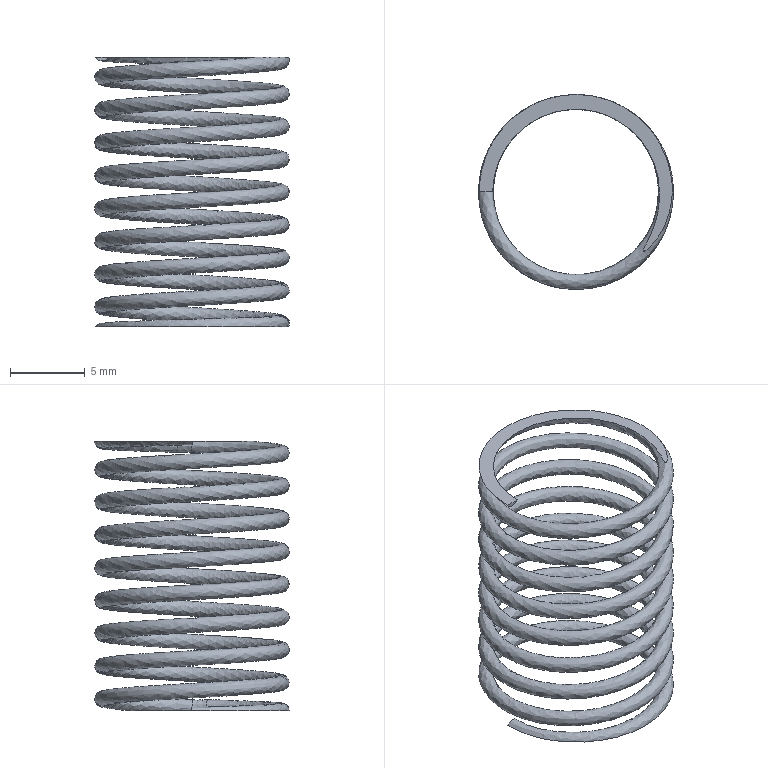Part | NX | features SPLINE_LAW 3, BRIDGE_CURVE 2, DATUM_CSYS 2, DATUM_PLANE 2, TRIM BODY 2, ABSOLUTE_DATUM_AXIS 1, ABSOLUTE_DATUM_PLANE 1, DATUM_ON_PATH 1, FLEXIBLE_PART 1, FSET 1, SKETCH 1, SKIN 1 | 1 solid | 9 faces | volume 252.111 mm3 | spline 5 | plane 4